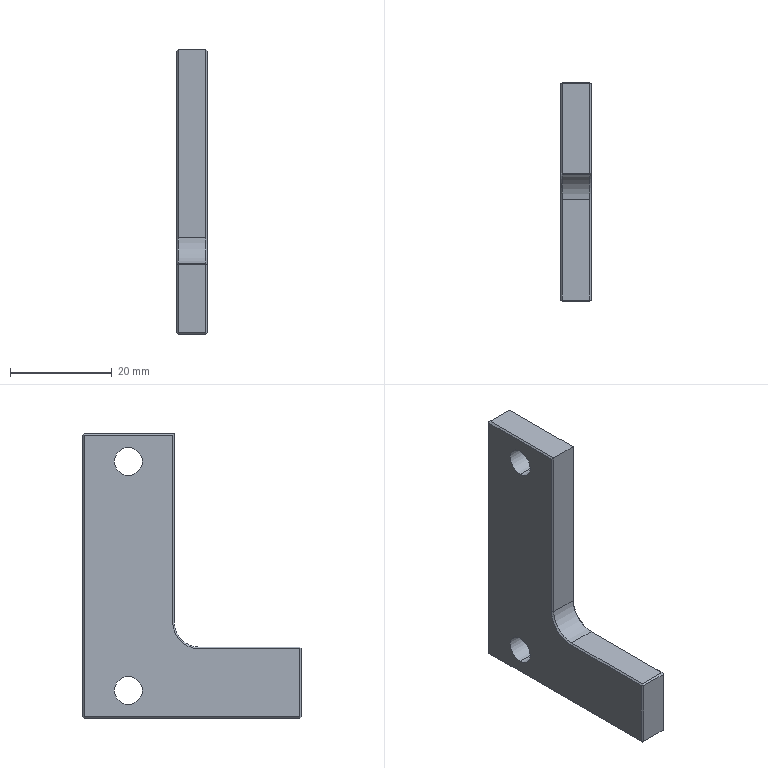Part | NX | 1 solid | 31 faces | box 6 x 43 x 56 mm | volume 7877 mm3 | plane 24 | cylinder 5 | cone 2 | commonest cylinder face diameters 5.5 x4 10 x1
STEP:
#1=CARTESIAN_POINT('',(2321.8,254.1,-75.2));
#2=VERTEX_POINT('',#1);
#3=CARTESIAN_POINT('',(2327.2,254.1,-75.2));
#4=VERTEX_POINT('',#3);
#5=CARTESIAN_POINT('',(2324.5,254.1,-75.2));
#6=DIRECTION('',(1.,0.,0.));
#7=VECTOR('',#6,1000.);
#8=LINE('',#5,#7);
#9=EDGE_CURVE('',#2,#4,#8,.T.);
#10=ORIENTED_EDGE('',*,*,#9,.T.);
#11=CARTESIAN_POINT('',(2327.2,211.7,-75.2));
#12=VERTEX_POINT('',#11);
#13=CARTESIAN_POINT('',(2327.2,232.9,-75.2));
#14=DIRECTION('',(0.,1.,0.));
#15=VECTOR('',#14,1000.);
#16=LINE('',#13,#15);
#17=EDGE_CURVE('',#12,#4,#16,.T.);
#18=ORIENTED_EDGE('',*,*,#17,.F.);
#19=CARTESIAN_POINT('',(2321.8,211.7,-75.2));
#20=VERTEX_POINT('',#19);
#21=CARTESIAN_POINT('',(2324.5,211.7,-75.2));
#22=DIRECTION('',(-1.,0.,0.));
#23=VECTOR('',#22,1000.);
#24=LINE('',#21,#23);
#25=EDGE_CURVE('',#12,#20,#24,.T.);
#26=ORIENTED_EDGE('',*,*,#25,.T.);
#27=CARTESIAN_POINT('',(2321.8,232.9,-75.2));
#28=DIRECTION('',(0.,1.,0.));
#29=VECTOR('',#28,1000.);
#30=LINE('',#27,#29);
#31=EDGE_CURVE('',#20,#2,#30,.T.);
#32=ORIENTED_EDGE('',*,*,#31,.T.);
#33=EDGE_LOOP('',(#10,#18,#26,#32));
#34=FACE_BOUND('',#33,.T.);
#35=CARTESIAN_POINT('',(2321.5,254.4,-75.2));
#36=DIRECTION('',(0.,0.,-1.));
#37=DIRECTION('',(-1.,0.,0.));
#38=AXIS2_PLACEMENT_3D('',#35,#36,#37);
#39=PLANE('',#38);
#40=ADVANCED_FACE('',(#34),#39,.T.);
#41=CARTESIAN_POINT('',(2321.8,254.4,-19.5));
#42=VERTEX_POINT('',#41);
#43=CARTESIAN_POINT('',(2327.2,254.4,-19.5));
#44=VERTEX_POINT('',#43);
#45=CARTESIAN_POINT('',(2324.5,254.4,-19.5));
#46=DIRECTION('',(1.,0.,0.));
#47=VECTOR('',#46,1000.);
#48=LINE('',#45,#47);
#49=EDGE_CURVE('',#42,#44,#48,.T.);
#50=ORIENTED_EDGE('',*,*,#49,.T.);
#51=CARTESIAN_POINT('',(2327.2,254.4,-74.9));
#52=VERTEX_POINT('',#51);
#53=CARTESIAN_POINT('',(2327.2,254.4,-47.2));
#54=DIRECTION('',(0.,0.,1.));
#55=VECTOR('',#54,1000.);
#56=LINE('',#53,#55);
#57=EDGE_CURVE('',#52,#44,#56,.T.);
#58=ORIENTED_EDGE('',*,*,#57,.F.);
#59=CARTESIAN_POINT('',(2321.8,254.4,-74.9));
#60=VERTEX_POINT('',#59);
#61=CARTESIAN_POINT('',(2324.5,254.4,-74.9));
#62=DIRECTION('',(1.,0.,0.));
#63=VECTOR('',#62,1000.);
#64=LINE('',#61,#63);
#65=EDGE_CURVE('',#60,#52,#64,.T.);
#66=ORIENTED_EDGE('',*,*,#65,.F.);
#67=CARTESIAN_POINT('',(2321.8,254.4,-47.2));
#68=DIRECTION('',(0.,0.,1.));
#69=VECTOR('',#68,1000.);
#70=LINE('',#67,#69);
#71=EDGE_CURVE('',#60,#42,#70,.T.);
#72=ORIENTED_EDGE('',*,*,#71,.T.);
#73=EDGE_LOOP('',(#50,#58,#66,#72));
#74=FACE_BOUND('',#73,.T.);
#75=CARTESIAN_POINT('',(2321.5,254.4,-19.2));
#76=DIRECTION('',(0.,1.,0.));
#77=DIRECTION('',(1.,0.,0.));
#78=AXIS2_PLACEMENT_3D('',#75,#76,#77);
#79=PLANE('',#78);
#80=ADVANCED_FACE('',(#74),#79,.T.);
#81=CARTESIAN_POINT('',(2321.8,254.1,-19.2));
#82=VERTEX_POINT('',#81);
#83=CARTESIAN_POINT('',(2321.8,236.4,-19.2));
#84=VERTEX_POINT('',#83);
#85=CARTESIAN_POINT('',(2321.8,245.4,-19.2));
#86=DIRECTION('',(0.,-1.,0.));
#87=VECTOR('',#86,1000.);
#88=LINE('',#85,#87);
#89=EDGE_CURVE('',#82,#84,#88,.T.);
#90=ORIENTED_EDGE('',*,*,#89,.T.);
#91=CARTESIAN_POINT('',(2327.2,236.4,-19.2));
#92=VERTEX_POINT('',#91);
#93=CARTESIAN_POINT('',(2321.5,236.4,-19.2));
#94=DIRECTION('',(1.,0.,0.));
#95=VECTOR('',#94,1000.);
#96=LINE('',#93,#95);
#97=EDGE_CURVE('',#84,#92,#96,.T.);
#98=ORIENTED_EDGE('',*,*,#97,.T.);
#99=CARTESIAN_POINT('',(2327.2,254.1,-19.2));
#100=VERTEX_POINT('',#99);
#101=CARTESIAN_POINT('',(2327.2,245.4,-19.2));
#102=DIRECTION('',(0.,-1.,0.));
#103=VECTOR('',#102,1000.);
#104=LINE('',#101,#103);
#105=EDGE_CURVE('',#100,#92,#104,.T.);
#106=ORIENTED_EDGE('',*,*,#105,.F.);
#107=CARTESIAN_POINT('',(2324.5,254.1,-19.2));
#108=DIRECTION('',(1.,0.,0.));
#109=VECTOR('',#108,1000.);
#110=LINE('',#107,#109);
#111=EDGE_CURVE('',#82,#100,#110,.T.);
#112=ORIENTED_EDGE('',*,*,#111,.F.);
#113=EDGE_LOOP('',(#90,#98,#106,#112));
#114=FACE_BOUND('',#113,.T.);
#115=CARTESIAN_POINT('',(2321.5,236.4,-19.2));
#116=DIRECTION('',(0.,0.,1.));
#117=DIRECTION('',(1.,0.,0.));
#118=AXIS2_PLACEMENT_3D('',#115,#116,#117);
#119=PLANE('',#118);
#120=ADVANCED_FACE('',(#114),#119,.T.);
#121=CARTESIAN_POINT('',(2327.2,236.4,-56.2));
#122=VERTEX_POINT('',#121);
#123=CARTESIAN_POINT('',(2321.8,236.4,-56.2));
#124=VERTEX_POINT('',#123);
#125=CARTESIAN_POINT('',(2321.5,236.4,-56.2));
#126=DIRECTION('',(-1.,0.,0.));
#127=VECTOR('',#126,1000.);
#128=LINE('',#125,#127);
#129=EDGE_CURVE('',#122,#124,#128,.T.);
#130=ORIENTED_EDGE('',*,*,#129,.F.);
#131=CARTESIAN_POINT('',(2327.2,236.4,-37.7));
#132=DIRECTION('',(0.,0.,-1.));
#133=VECTOR('',#132,1000.);
#134=LINE('',#131,#133);
#135=EDGE_CURVE('',#92,#122,#134,.T.);
#136=ORIENTED_EDGE('',*,*,#135,.F.);
#137=ORIENTED_EDGE('',*,*,#97,.F.);
#138=CARTESIAN_POINT('',(2321.8,236.4,-37.7));
#139=DIRECTION('',(0.,0.,-1.));
#140=VECTOR('',#139,1000.);
#141=LINE('',#138,#140);
#142=EDGE_CURVE('',#84,#124,#141,.T.);
#143=ORIENTED_EDGE('',*,*,#142,.T.);
#144=EDGE_LOOP('',(#130,#136,#137,#143));
#145=FACE_BOUND('',#144,.T.);
#146=CARTESIAN_POINT('',(2321.5,236.4,-75.2));
#147=DIRECTION('',(0.,-1.,0.));
#148=DIRECTION('',(0.,0.,-1.));
#149=AXIS2_PLACEMENT_3D('',#146,#147,#148);
#150=PLANE('',#149);
#151=ADVANCED_FACE('',(#145),#150,.T.);
#152=CARTESIAN_POINT('',(2327.2,211.4,-74.9));
#153=VERTEX_POINT('',#152);
#154=CARTESIAN_POINT('',(2321.8,211.4,-74.9));
#155=VERTEX_POINT('',#154);
#156=CARTESIAN_POINT('',(2324.5,211.4,-74.9));
#157=DIRECTION('',(-1.,0.,0.));
#158=VECTOR('',#157,1000.);
#159=LINE('',#156,#158);
#160=EDGE_CURVE('',#153,#155,#159,.T.);
#161=ORIENTED_EDGE('',*,*,#160,.F.);
#162=CARTESIAN_POINT('',(2327.2,211.4,-61.5));
#163=VERTEX_POINT('',#162);
#164=CARTESIAN_POINT('',(2327.2,211.4,-68.2));
#165=DIRECTION('',(0.,0.,-1.));
#166=VECTOR('',#165,1000.);
#167=LINE('',#164,#166);
#168=EDGE_CURVE('',#163,#153,#167,.T.);
#169=ORIENTED_EDGE('',*,*,#168,.F.);
#170=CARTESIAN_POINT('',(2321.8,211.4,-61.5));
#171=VERTEX_POINT('',#170);
#172=CARTESIAN_POINT('',(2324.5,211.4,-61.5));
#173=DIRECTION('',(1.,0.,0.));
#174=VECTOR('',#173,1000.);
#175=LINE('',#172,#174);
#176=EDGE_CURVE('',#171,#163,#175,.T.);
#177=ORIENTED_EDGE('',*,*,#176,.F.);
#178=CARTESIAN_POINT('',(2321.8,211.4,-68.2));
#179=DIRECTION('',(0.,0.,-1.));
#180=VECTOR('',#179,1000.);
#181=LINE('',#178,#180);
#182=EDGE_CURVE('',#171,#155,#181,.T.);
#183=ORIENTED_EDGE('',*,*,#182,.T.);
#184=EDGE_LOOP('',(#161,#169,#177,#183));
#185=FACE_BOUND('',#184,.T.);
#186=CARTESIAN_POINT('',(2325.077,211.4,-68.526));
#187=DIRECTION('',(0.,-1.,0.));
#188=DIRECTION('',(0.,0.,-1.));
#189=AXIS2_PLACEMENT_3D('',#186,#187,#188);
#190=PLANE('',#189);
#191=ADVANCED_FACE('',(#185),#190,.T.);
#192=CARTESIAN_POINT('',(2321.8,231.4,-61.2));
#193=VERTEX_POINT('',#192);
#194=CARTESIAN_POINT('',(2321.8,211.7,-61.2));
#195=VERTEX_POINT('',#194);
#196=CARTESIAN_POINT('',(2321.8,221.4,-61.2));
#197=DIRECTION('',(0.,-1.,0.));
#198=VECTOR('',#197,1000.);
#199=LINE('',#196,#198);
#200=EDGE_CURVE('',#193,#195,#199,.T.);
#201=ORIENTED_EDGE('',*,*,#200,.T.);
#202=CARTESIAN_POINT('',(2327.2,211.7,-61.2));
#203=VERTEX_POINT('',#202);
#204=CARTESIAN_POINT('',(2324.5,211.7,-61.2));
#205=DIRECTION('',(1.,0.,0.));
#206=VECTOR('',#205,1000.);
#207=LINE('',#204,#206);
#208=EDGE_CURVE('',#195,#203,#207,.T.);
#209=ORIENTED_EDGE('',*,*,#208,.T.);
#210=CARTESIAN_POINT('',(2327.2,231.4,-61.2));
#211=VERTEX_POINT('',#210);
#212=CARTESIAN_POINT('',(2327.2,221.4,-61.2));
#213=DIRECTION('',(0.,-1.,0.));
#214=VECTOR('',#213,1000.);
#215=LINE('',#212,#214);
#216=EDGE_CURVE('',#211,#203,#215,.T.);
#217=ORIENTED_EDGE('',*,*,#216,.F.);
#218=CARTESIAN_POINT('',(2321.5,231.4,-61.2));
#219=DIRECTION('',(-1.,0.,0.));
#220=VECTOR('',#219,1000.);
#221=LINE('',#218,#220);
#222=EDGE_CURVE('',#211,#193,#221,.T.);
#223=ORIENTED_EDGE('',*,*,#222,.T.);
#224=EDGE_LOOP('',(#201,#209,#217,#223));
#225=FACE_BOUND('',#224,.T.);
#226=CARTESIAN_POINT('',(2321.5,236.4,-61.2));
#227=DIRECTION('',(0.,0.,1.));
#228=DIRECTION('',(1.,0.,0.));
#229=AXIS2_PLACEMENT_3D('',#226,#227,#228);
#230=PLANE('',#229);
#231=ADVANCED_FACE('',(#225),#230,.T.);
#232=CARTESIAN_POINT('',(2321.8,231.4,-56.2));
#233=DIRECTION('',(-1.,0.,0.));
#234=DIRECTION('',(0.,0.,-1.));
#235=AXIS2_PLACEMENT_3D('',#232,#233,#234);
#236=CIRCLE('',#235,5.);
#237=EDGE_CURVE('',#124,#193,#236,.T.);
#238=ORIENTED_EDGE('',*,*,#237,.T.);
#239=ORIENTED_EDGE('',*,*,#222,.F.);
#240=CARTESIAN_POINT('',(2327.2,231.4,-56.2));
#241=DIRECTION('',(-1.,0.,0.));
#242=DIRECTION('',(0.,0.,-1.));
#243=AXIS2_PLACEMENT_3D('',#240,#241,#242);
#244=CIRCLE('',#243,5.);
#245=EDGE_CURVE('',#122,#211,#244,.T.);
#246=ORIENTED_EDGE('',*,*,#245,.F.);
#247=ORIENTED_EDGE('',*,*,#129,.T.);
#248=EDGE_LOOP('',(#238,#239,#246,#247));
#249=FACE_BOUND('',#248,.T.);
#250=CARTESIAN_POINT('',(2321.5,231.4,-56.2));
#251=DIRECTION('',(-1.,0.,0.));
#252=DIRECTION('',(0.,0.,-1.));
#253=AXIS2_PLACEMENT_3D('',#250,#251,#252);
#254=CYLINDRICAL_SURFACE('',#253,5.);
#255=ADVANCED_FACE('',(#249),#254,.F.);
#256=ORIENTED_EDGE('',*,*,#49,.F.);
#257=CARTESIAN_POINT('',(2321.65,254.25,-19.35));
#258=VERTEX_POINT('',#257);
#259=CARTESIAN_POINT('',(2347.565,280.165,-45.265));
#260=DIRECTION('',(0.5774,0.5774,-0.5774));
#261=VECTOR('',#260,1000.);
#262=LINE('',#259,#261);
#263=EDGE_CURVE('',#258,#42,#262,.T.);
#264=ORIENTED_EDGE('',*,*,#263,.F.);
#265=CARTESIAN_POINT('',(2295.735,280.165,-45.265));
#266=DIRECTION('',(0.5774,-0.5774,0.5774));
#267=VECTOR('',#266,1000.);
#268=LINE('',#265,#267);
#269=EDGE_CURVE('',#258,#82,#268,.T.);
#270=ORIENTED_EDGE('',*,*,#269,.T.);
#271=ORIENTED_EDGE('',*,*,#111,.T.);
#272=CARTESIAN_POINT('',(2327.35,254.25,-19.35));
#273=VERTEX_POINT('',#272);
#274=CARTESIAN_POINT('',(2353.265,280.165,-45.265));
#275=DIRECTION('',(-0.5774,-0.5774,0.5774));
#276=VECTOR('',#275,1000.);
#277=LINE('',#274,#276);
#278=EDGE_CURVE('',#273,#100,#277,.T.);
#279=ORIENTED_EDGE('',*,*,#278,.F.);
#280=CARTESIAN_POINT('',(2301.435,280.165,-45.265));
#281=DIRECTION('',(-0.5774,0.5774,-0.5774));
#282=VECTOR('',#281,1000.);
#283=LINE('',#280,#282);
#284=EDGE_CURVE('',#273,#44,#283,.T.);
#285=ORIENTED_EDGE('',*,*,#284,.T.);
#286=EDGE_LOOP('',(#256,#264,#270,#271,#279,#285));
#287=FACE_BOUND('',#286,.T.);
#288=CARTESIAN_POINT('',(2324.5,254.25,-19.35));
#289=DIRECTION('',(0.,0.7071,0.7071));
#290=DIRECTION('',(1.,0.,0.));
#291=AXIS2_PLACEMENT_3D('',#288,#289,#290);
#292=PLANE('',#291);
#293=ADVANCED_FACE('',(#287),#292,.T.);
#294=ORIENTED_EDGE('',*,*,#9,.F.);
#295=CARTESIAN_POINT('',(2321.65,254.25,-75.05));
#296=VERTEX_POINT('',#295);
#297=CARTESIAN_POINT('',(2329.326,246.574,-82.726));
#298=DIRECTION('',(0.5774,-0.5774,-0.5774));
#299=VECTOR('',#298,1000.);
#300=LINE('',#297,#299);
#301=EDGE_CURVE('',#296,#2,#300,.T.);
#302=ORIENTED_EDGE('',*,*,#301,.F.);
#303=CARTESIAN_POINT('',(2321.5,254.1,-75.2));
#304=DIRECTION('',(0.5774,0.5774,0.5774));
#305=VECTOR('',#304,1000.);
#306=LINE('',#303,#305);
#307=EDGE_CURVE('',#296,#60,#306,.T.);
#308=ORIENTED_EDGE('',*,*,#307,.T.);
#309=ORIENTED_EDGE('',*,*,#65,.T.);
#310=CARTESIAN_POINT('',(2327.35,254.25,-75.05));
#311=VERTEX_POINT('',#310);
#312=CARTESIAN_POINT('',(2321.5,260.1,-69.2));
#313=DIRECTION('',(-0.5774,0.5774,0.5774));
#314=VECTOR('',#313,1000.);
#315=LINE('',#312,#314);
#316=EDGE_CURVE('',#311,#52,#315,.T.);
#317=ORIENTED_EDGE('',*,*,#316,.F.);
#318=CARTESIAN_POINT('',(2319.674,246.574,-82.726));
#319=DIRECTION('',(-0.5774,-0.5774,-0.5774));
#320=VECTOR('',#319,1000.);
#321=LINE('',#318,#320);
#322=EDGE_CURVE('',#311,#4,#321,.T.);
#323=ORIENTED_EDGE('',*,*,#322,.T.);
#324=EDGE_LOOP('',(#294,#302,#308,#309,#317,#323));
#325=FACE_BOUND('',#324,.T.);
#326=CARTESIAN_POINT('',(2324.5,254.25,-75.05));
#327=DIRECTION('',(0.,0.7071,-0.7071));
#328=DIRECTION('',(-1.,0.,0.));
#329=AXIS2_PLACEMENT_3D('',#326,#327,#328);
#330=PLANE('',#329);
#331=ADVANCED_FACE('',(#325),#330,.T.);
#332=ORIENTED_EDGE('',*,*,#168,.T.);
#333=CARTESIAN_POINT('',(2327.35,211.55,-75.05));
#334=VERTEX_POINT('',#333);
#335=CARTESIAN_POINT('',(2297.565,181.765,-45.265));
#336=DIRECTION('',(0.5774,0.5774,-0.5774));
#337=VECTOR('',#336,1000.);
#338=LINE('',#335,#337);
#339=EDGE_CURVE('',#153,#334,#338,.T.);
#340=ORIENTED_EDGE('',*,*,#339,.T.);
#341=CARTESIAN_POINT('',(2327.5,211.7,-74.9));
#342=VERTEX_POINT('',#341);
#343=CARTESIAN_POINT('',(2357.135,241.335,-45.265));
#344=DIRECTION('',(0.5774,0.5774,0.5774));
#345=VECTOR('',#344,1000.);
#346=LINE('',#343,#345);
#347=EDGE_CURVE('',#334,#342,#346,.T.);
#348=ORIENTED_EDGE('',*,*,#347,.T.);
#349=CARTESIAN_POINT('',(2327.5,211.7,-61.5));
#350=VERTEX_POINT('',#349);
#351=CARTESIAN_POINT('',(2327.5,211.7,-68.2));
#352=DIRECTION('',(0.,0.,-1.));
#353=VECTOR('',#352,1000.);
#354=LINE('',#351,#353);
#355=EDGE_CURVE('',#350,#342,#354,.T.);
#356=ORIENTED_EDGE('',*,*,#355,.F.);
#357=CARTESIAN_POINT('',(2327.35,211.55,-61.35));
#358=VERTEX_POINT('',#357);
#359=CARTESIAN_POINT('',(2311.265,195.465,-45.265));
#360=DIRECTION('',(0.5774,0.5774,-0.5774));
#361=VECTOR('',#360,1000.);
#362=LINE('',#359,#361);
#363=EDGE_CURVE('',#358,#350,#362,.T.);
#364=ORIENTED_EDGE('',*,*,#363,.F.);
#365=CARTESIAN_POINT('',(2343.435,227.635,-45.265));
#366=DIRECTION('',(-0.5774,-0.5774,-0.5774));
#367=VECTOR('',#366,1000.);
#368=LINE('',#365,#367);
#369=EDGE_CURVE('',#358,#163,#368,.T.);
#370=ORIENTED_EDGE('',*,*,#369,.T.);
#371=EDGE_LOOP('',(#332,#340,#348,#356,#364,#370));
#372=FACE_BOUND('',#371,.T.);
#373=CARTESIAN_POINT('',(2327.35,211.55,-68.2));
#374=DIRECTION('',(-0.7071,0.7071,0.));
#375=DIRECTION('',(0.,0.,1.));
#376=AXIS2_PLACEMENT_3D('',#373,#374,#375);
#377=PLANE('',#376);
#378=ADVANCED_FACE('',(#372),#377,.F.);
#379=ORIENTED_EDGE('',*,*,#245,.T.);
#380=CARTESIAN_POINT('',(2327.5,231.4,-61.5));
#381=VERTEX_POINT('',#380);
#382=CARTESIAN_POINT('',(2327.5,231.4,-61.5));
#383=DIRECTION('',(-0.7071,0.,0.7071));
#384=VECTOR('',#383,1000.);
#385=LINE('',#382,#384);
#386=EDGE_CURVE('',#381,#211,#385,.T.);
#387=ORIENTED_EDGE('',*,*,#386,.F.);
#388=CARTESIAN_POINT('',(2327.5,236.7,-56.2));
#389=VERTEX_POINT('',#388);
#390=CARTESIAN_POINT('',(2327.5,231.4,-56.2));
#391=DIRECTION('',(-1.,0.,0.));
#392=DIRECTION('',(0.,0.,-1.));
#393=AXIS2_PLACEMENT_3D('',#390,#391,#392);
#394=CIRCLE('',#393,5.3);
#395=EDGE_CURVE('',#389,#381,#394,.T.);
#396=ORIENTED_EDGE('',*,*,#395,.F.);
#397=CARTESIAN_POINT('',(2327.2,236.4,-56.2));
#398=DIRECTION('',(0.7071,0.7071,0.));
#399=VECTOR('',#398,1000.);
#400=LINE('',#397,#399);
#401=EDGE_CURVE('',#122,#389,#400,.T.);
#402=ORIENTED_EDGE('',*,*,#401,.F.);
#403=EDGE_LOOP('',(#379,#387,#396,#402));
#404=FACE_BOUND('',#403,.T.);
#405=CARTESIAN_POINT('',(2327.2,231.4,-56.2));
#406=DIRECTION('',(1.,0.,0.));
#407=DIRECTION('',(0.,-1.,0.));
#408=AXIS2_PLACEMENT_3D('',#405,#406,#407);
#409=CONICAL_SURFACE('',#408,5.,0.7854);
#410=ADVANCED_FACE('',(#404),#409,.F.);
#411=ORIENTED_EDGE('',*,*,#200,.F.);
#412=CARTESIAN_POINT('',(2321.5,231.4,-61.5));
#413=VERTEX_POINT('',#412);
#414=CARTESIAN_POINT('',(2321.8,231.4,-61.2));
#415=DIRECTION('',(-0.7071,0.,-0.7071));
#416=VECTOR('',#415,1000.);
#417=LINE('',#414,#416);
#418=EDGE_CURVE('',#193,#413,#417,.T.);
#419=ORIENTED_EDGE('',*,*,#418,.T.);
#420=CARTESIAN_POINT('',(2321.5,211.7,-61.5));
#421=VERTEX_POINT('',#420);
#422=CARTESIAN_POINT('',(2321.5,221.4,-61.5));
#423=DIRECTION('',(0.,-1.,0.));
#424=VECTOR('',#423,1000.);
#425=LINE('',#422,#424);
#426=EDGE_CURVE('',#413,#421,#425,.T.);
#427=ORIENTED_EDGE('',*,*,#426,.T.);
#428=CARTESIAN_POINT('',(2321.65,211.55,-61.35));
#429=VERTEX_POINT('',#428);
#430=CARTESIAN_POINT('',(2337.735,195.465,-45.265));
#431=DIRECTION('',(0.5774,-0.5774,0.5774));
#432=VECTOR('',#431,1000.);
#433=LINE('',#430,#432);
#434=EDGE_CURVE('',#421,#429,#433,.T.);
#435=ORIENTED_EDGE('',*,*,#434,.T.);
#436=CARTESIAN_POINT('',(2337.735,227.635,-45.265));
#437=DIRECTION('',(-0.5774,-0.5774,-0.5774));
#438=VECTOR('',#437,1000.);
#439=LINE('',#436,#438);
#440=EDGE_CURVE('',#195,#429,#439,.T.);
#441=ORIENTED_EDGE('',*,*,#440,.F.);
#442=EDGE_LOOP('',(#411,#419,#427,#435,#441));
#443=FACE_BOUND('',#442,.T.);
#444=CARTESIAN_POINT('',(2321.65,221.4,-61.35));
#445=DIRECTION('',(-0.7071,0.,0.7071));
#446=DIRECTION('',(0.,1.,0.));
#447=AXIS2_PLACEMENT_3D('',#444,#445,#446);
#448=PLANE('',#447);
#449=ADVANCED_FACE('',(#443),#448,.T.);
#450=ORIENTED_EDGE('',*,*,#237,.F.);
#451=CARTESIAN_POINT('',(2321.5,236.7,-56.2));
#452=VERTEX_POINT('',#451);
#453=CARTESIAN_POINT('',(2321.8,236.4,-56.2));
#454=DIRECTION('',(-0.7071,0.7071,0.));
#455=VECTOR('',#454,1000.);
#456=LINE('',#453,#455);
#457=EDGE_CURVE('',#124,#452,#456,.T.);
#458=ORIENTED_EDGE('',*,*,#457,.T.);
#459=CARTESIAN_POINT('',(2321.5,231.4,-56.2));
#460=DIRECTION('',(-1.,0.,0.));
#461=DIRECTION('',(0.,0.,-1.));
#462=AXIS2_PLACEMENT_3D('',#459,#460,#461);
#463=CIRCLE('',#462,5.3);
#464=EDGE_CURVE('',#452,#413,#463,.T.);
#465=ORIENTED_EDGE('',*,*,#464,.T.);
#466=ORIENTED_EDGE('',*,*,#418,.F.);
#467=EDGE_LOOP('',(#450,#458,#465,#466));
#468=FACE_BOUND('',#467,.T.);
#469=CARTESIAN_POINT('',(2321.8,231.4,-56.2));
#470=DIRECTION('',(-1.,0.,0.));
#471=DIRECTION('',(0.,1.,0.));
#472=AXIS2_PLACEMENT_3D('',#469,#470,#471);
#473=CONICAL_SURFACE('',#472,5.,0.7854);
#474=ADVANCED_FACE('',(#468),#473,.F.);
#475=ORIENTED_EDGE('',*,*,#176,.T.);
#476=ORIENTED_EDGE('',*,*,#369,.F.);
#477=CARTESIAN_POINT('',(2311.265,227.635,-45.265));
#478=DIRECTION('',(-0.5774,0.5774,0.5774));
#479=VECTOR('',#478,1000.);
#480=LINE('',#477,#479);
#481=EDGE_CURVE('',#358,#203,#480,.T.);
#482=ORIENTED_EDGE('',*,*,#481,.T.);
#483=ORIENTED_EDGE('',*,*,#208,.F.);
#484=ORIENTED_EDGE('',*,*,#440,.T.);
#485=CARTESIAN_POINT('',(2305.565,227.635,-45.265));
#486=DIRECTION('',(-0.5774,0.5774,0.5774));
#487=VECTOR('',#486,1000.);
#488=LINE('',#485,#487);
#489=EDGE_CURVE('',#171,#429,#488,.T.);
#490=ORIENTED_EDGE('',*,*,#489,.F.);
#491=EDGE_LOOP('',(#475,#476,#482,#483,#484,#490));
#492=FACE_BOUND('',#491,.T.);
#493=CARTESIAN_POINT('',(2324.5,211.55,-61.35));
#494=DIRECTION('',(0.,0.7071,-0.7071));
#495=DIRECTION('',(-1.,0.,0.));
#496=AXIS2_PLACEMENT_3D('',#493,#494,#495);
#497=PLANE('',#496);
#498=ADVANCED_FACE('',(#492),#497,.F.);
#499=ORIENTED_EDGE('',*,*,#182,.F.);
#500=ORIENTED_EDGE('',*,*,#489,.T.);
#501=ORIENTED_EDGE('',*,*,#434,.F.);
#502=CARTESIAN_POINT('',(2321.5,211.7,-74.9));
#503=VERTEX_POINT('',#502);
#504=CARTESIAN_POINT('',(2321.5,211.7,-68.2));
#505=DIRECTION('',(0.,0.,-1.));
#506=VECTOR('',#505,1000.);
#507=LINE('',#504,#506);
#508=EDGE_CURVE('',#421,#503,#507,.T.);
#509=ORIENTED_EDGE('',*,*,#508,.T.);
#510=CARTESIAN_POINT('',(2321.65,211.55,-75.05));
#511=VERTEX_POINT('',#510);
#512=CARTESIAN_POINT('',(2291.865,241.335,-45.265));
#513=DIRECTION('',(-0.5774,0.5774,0.5774));
#514=VECTOR('',#513,1000.);
#515=LINE('',#512,#514);
#516=EDGE_CURVE('',#511,#503,#515,.T.);
#517=ORIENTED_EDGE('',*,*,#516,.F.);
#518=CARTESIAN_POINT('',(2351.435,181.765,-45.265));
#519=DIRECTION('',(-0.5774,0.5774,-0.5774));
#520=VECTOR('',#519,1000.);
#521=LINE('',#518,#520);
#522=EDGE_CURVE('',#155,#511,#521,.T.);
#523=ORIENTED_EDGE('',*,*,#522,.F.);
#524=EDGE_LOOP('',(#499,#500,#501,#509,#517,#523));
#525=FACE_BOUND('',#524,.T.);
#526=CARTESIAN_POINT('',(2321.65,211.55,-68.2));
#527=DIRECTION('',(-0.7071,-0.7071,0.));
#528=DIRECTION('',(-0.7071,0.7071,0.));
#529=AXIS2_PLACEMENT_3D('',#526,#527,#528);
#530=PLANE('',#529);
#531=ADVANCED_FACE('',(#525),#530,.T.);
#532=ORIENTED_EDGE('',*,*,#160,.T.);
#533=ORIENTED_EDGE('',*,*,#522,.T.);
#534=CARTESIAN_POINT('',(2291.865,181.765,-45.265));
#535=DIRECTION('',(-0.5774,-0.5774,0.5774));
#536=VECTOR('',#535,1000.);
#537=LINE('',#534,#536);
#538=EDGE_CURVE('',#20,#511,#537,.T.);
#539=ORIENTED_EDGE('',*,*,#538,.F.);
#540=ORIENTED_EDGE('',*,*,#25,.F.);
#541=CARTESIAN_POINT('',(2357.135,181.765,-45.265));
#542=DIRECTION('',(0.5774,-0.5774,0.5774));
#543=VECTOR('',#542,1000.);
#544=LINE('',#541,#543);
#545=EDGE_CURVE('',#12,#334,#544,.T.);
#546=ORIENTED_EDGE('',*,*,#545,.T.);
#547=ORIENTED_EDGE('',*,*,#339,.F.);
#548=EDGE_LOOP('',(#532,#533,#539,#540,#546,#547));
#549=FACE_BOUND('',#548,.T.);
#550=CARTESIAN_POINT('',(2324.5,211.55,-75.05));
#551=DIRECTION('',(0.,0.7071,0.7071));
#552=DIRECTION('',(1.,0.,0.));
#553=AXIS2_PLACEMENT_3D('',#550,#551,#552);
#554=PLANE('',#553);
#555=ADVANCED_FACE('',(#549),#554,.F.);
#556=CARTESIAN_POINT('',(2327.5,236.7,-19.5));
#557=VERTEX_POINT('',#556);
#558=CARTESIAN_POINT('',(2327.5,236.7,-37.7));
#559=DIRECTION('',(0.,0.,-1.));
#560=VECTOR('',#559,1000.);
#561=LINE('',#558,#560);
#562=EDGE_CURVE('',#557,#389,#561,.T.);
#563=ORIENTED_EDGE('',*,*,#562,.T.);
#564=ORIENTED_EDGE('',*,*,#395,.T.);
#565=CARTESIAN_POINT('',(2327.5,221.4,-61.5));
#566=DIRECTION('',(0.,-1.,0.));
#567=VECTOR('',#566,1000.);
#568=LINE('',#565,#567);
#569=EDGE_CURVE('',#381,#350,#568,.T.);
#570=ORIENTED_EDGE('',*,*,#569,.T.);
#571=ORIENTED_EDGE('',*,*,#355,.T.);
#572=CARTESIAN_POINT('',(2327.5,254.1,-74.9));
#573=VERTEX_POINT('',#572);
#574=CARTESIAN_POINT('',(2327.5,232.9,-74.9));
#575=DIRECTION('',(0.,1.,0.));
#576=VECTOR('',#575,1000.);
#577=LINE('',#574,#576);
#578=EDGE_CURVE('',#342,#573,#577,.T.);
#579=ORIENTED_EDGE('',*,*,#578,.T.);
#580=CARTESIAN_POINT('',(2327.5,254.1,-19.5));
#581=VERTEX_POINT('',#580);
#582=CARTESIAN_POINT('',(2327.5,254.1,-47.2));
#583=DIRECTION('',(0.,0.,1.));
#584=VECTOR('',#583,1000.);
#585=LINE('',#582,#584);
#586=EDGE_CURVE('',#573,#581,#585,.T.);
#587=ORIENTED_EDGE('',*,*,#586,.T.);
#588=CARTESIAN_POINT('',(2327.5,245.4,-19.5));
#589=DIRECTION('',(0.,-1.,0.));
#590=VECTOR('',#589,1000.);
#591=LINE('',#588,#590);
#592=EDGE_CURVE('',#581,#557,#591,.T.);
#593=ORIENTED_EDGE('',*,*,#592,.T.);
#594=EDGE_LOOP('',(#563,#564,#570,#571,#579,#587,#593));
#595=FACE_BOUND('',#594,.T.);
#596=CARTESIAN_POINT('',(2327.5,245.4,-66.95));
#597=VERTEX_POINT('',#596);
#598=CARTESIAN_POINT('',(2327.5,245.4,-72.45));
#599=VERTEX_POINT('',#598);
#600=CARTESIAN_POINT('',(2327.5,245.4,-69.7));
#601=DIRECTION('',(1.,0.,0.));
#602=DIRECTION('',(0.,0.,-1.));
#603=AXIS2_PLACEMENT_3D('',#600,#601,#602);
#604=CIRCLE('',#603,2.75);
#605=EDGE_CURVE('',#597,#599,#604,.T.);
#606=ORIENTED_EDGE('',*,*,#605,.F.);
#607=CARTESIAN_POINT('',(2327.5,245.4,-69.7));
#608=DIRECTION('',(1.,0.,0.));
#609=DIRECTION('',(0.,0.,-1.));
#610=AXIS2_PLACEMENT_3D('',#607,#608,#609);
#611=CIRCLE('',#610,2.75);
#612=EDGE_CURVE('',#599,#597,#611,.T.);
#613=ORIENTED_EDGE('',*,*,#612,.F.);
#614=EDGE_LOOP('',(#606,#613));
#615=FACE_BOUND('',#614,.T.);
#616=CARTESIAN_POINT('',(2327.5,245.4,-27.45));
#617=VERTEX_POINT('',#616);
#618=CARTESIAN_POINT('',(2327.5,245.4,-21.95));
#619=VERTEX_POINT('',#618);
#620=CARTESIAN_POINT('',(2327.5,245.4,-24.7));
#621=DIRECTION('',(1.,0.,0.));
#622=DIRECTION('',(0.,0.,-1.));
#623=AXIS2_PLACEMENT_3D('',#620,#621,#622);
#624=CIRCLE('',#623,2.75);
#625=EDGE_CURVE('',#617,#619,#624,.T.);
#626=ORIENTED_EDGE('',*,*,#625,.F.);
#627=CARTESIAN_POINT('',(2327.5,245.4,-24.7));
#628=DIRECTION('',(1.,0.,0.));
#629=DIRECTION('',(0.,0.,-1.));
#630=AXIS2_PLACEMENT_3D('',#627,#628,#629);
#631=CIRCLE('',#630,2.75);
#632=EDGE_CURVE('',#619,#617,#631,.T.);
#633=ORIENTED_EDGE('',*,*,#632,.F.);
#634=EDGE_LOOP('',(#626,#633));
#635=FACE_BOUND('',#634,.T.);
#636=CARTESIAN_POINT('',(2327.5,246.574,-45.265));
#637=DIRECTION('',(1.,0.,0.));
#638=DIRECTION('',(0.,1.,0.));
#639=AXIS2_PLACEMENT_3D('',#636,#637,#638);
#640=PLANE('',#639);
#641=ADVANCED_FACE('',(#595,#615,#635),#640,.T.);
#642=ORIENTED_EDGE('',*,*,#625,.T.);
#643=CARTESIAN_POINT('',(2321.5,245.4,-21.95));
#644=VERTEX_POINT('',#643);
#645=CARTESIAN_POINT('',(2320.9,245.4,-21.95));
#646=DIRECTION('',(1.,0.,0.));
#647=VECTOR('',#646,1000.);
#648=LINE('',#645,#647);
#649=EDGE_CURVE('',#644,#619,#648,.T.);
#650=ORIENTED_EDGE('',*,*,#649,.F.);
#651=CARTESIAN_POINT('',(2321.5,245.4,-27.45));
#652=VERTEX_POINT('',#651);
#653=CARTESIAN_POINT('',(2321.5,245.4,-24.7));
#654=DIRECTION('',(1.,0.,0.));
#655=DIRECTION('',(0.,0.,-1.));
#656=AXIS2_PLACEMENT_3D('',#653,#654,#655);
#657=CIRCLE('',#656,2.75);
#658=EDGE_CURVE('',#652,#644,#657,.T.);
#659=ORIENTED_EDGE('',*,*,#658,.F.);
#660=CARTESIAN_POINT('',(2320.9,245.4,-27.45));
#661=DIRECTION('',(1.,0.,0.));
#662=VECTOR('',#661,1000.);
#663=LINE('',#660,#662);
#664=EDGE_CURVE('',#652,#617,#663,.T.);
#665=ORIENTED_EDGE('',*,*,#664,.T.);
#666=EDGE_LOOP('',(#642,#650,#659,#665));
#667=FACE_BOUND('',#666,.T.);
#668=CARTESIAN_POINT('',(2320.9,245.4,-24.7));
#669=DIRECTION('',(1.,0.,0.));
#670=DIRECTION('',(0.,0.,-1.));
#671=AXIS2_PLACEMENT_3D('',#668,#669,#670);
#672=CYLINDRICAL_SURFACE('',#671,2.75);
#673=ADVANCED_FACE('',(#667),#672,.F.);
#674=CARTESIAN_POINT('',(2321.5,245.4,-66.95));
#675=VERTEX_POINT('',#674);
#676=CARTESIAN_POINT('',(2321.5,245.4,-72.45));
#677=VERTEX_POINT('',#676);
#678=CARTESIAN_POINT('',(2321.5,245.4,-69.7));
#679=DIRECTION('',(1.,0.,0.));
#680=DIRECTION('',(0.,0.,-1.));
#681=AXIS2_PLACEMENT_3D('',#678,#679,#680);
#682=CIRCLE('',#681,2.75);
#683=EDGE_CURVE('',#675,#677,#682,.T.);
#684=ORIENTED_EDGE('',*,*,#683,.F.);
#685=CARTESIAN_POINT('',(2320.9,245.4,-66.95));
#686=DIRECTION('',(1.,0.,0.));
#687=VECTOR('',#686,1000.);
#688=LINE('',#685,#687);
#689=EDGE_CURVE('',#675,#597,#688,.T.);
#690=ORIENTED_EDGE('',*,*,#689,.T.);
#691=ORIENTED_EDGE('',*,*,#605,.T.);
#692=CARTESIAN_POINT('',(2320.9,245.4,-72.45));
#693=DIRECTION('',(1.,0.,0.));
#694=VECTOR('',#693,1000.);
#695=LINE('',#692,#694);
#696=EDGE_CURVE('',#677,#599,#695,.T.);
#697=ORIENTED_EDGE('',*,*,#696,.F.);
#698=EDGE_LOOP('',(#684,#690,#691,#697));
#699=FACE_BOUND('',#698,.T.);
#700=CARTESIAN_POINT('',(2320.9,245.4,-69.7));
#701=DIRECTION('',(1.,0.,0.));
#702=DIRECTION('',(0.,0.,-1.));
#703=AXIS2_PLACEMENT_3D('',#700,#701,#702);
#704=CYLINDRICAL_SURFACE('',#703,2.75);
#705=ADVANCED_FACE('',(#699),#704,.F.);
#706=ORIENTED_EDGE('',*,*,#592,.F.);
#707=CARTESIAN_POINT('',(2353.265,228.335,-45.265));
#708=DIRECTION('',(-0.5774,0.5774,0.5774));
#709=VECTOR('',#708,1000.);
#710=LINE('',#707,#709);
#711=EDGE_CURVE('',#581,#273,#710,.T.);
#712=ORIENTED_EDGE('',*,*,#711,.T.);
#713=ORIENTED_EDGE('',*,*,#278,.T.);
#714=ORIENTED_EDGE('',*,*,#105,.T.);
#715=CARTESIAN_POINT('',(2353.265,262.465,-45.265));
#716=DIRECTION('',(0.5774,0.5774,-0.5774));
#717=VECTOR('',#716,1000.);
#718=LINE('',#715,#717);
#719=EDGE_CURVE('',#92,#557,#718,.T.);
#720=ORIENTED_EDGE('',*,*,#719,.T.);
#721=EDGE_LOOP('',(#706,#712,#713,#714,#720));
#722=FACE_BOUND('',#721,.T.);
#723=CARTESIAN_POINT('',(2327.35,245.4,-19.35));
#724=DIRECTION('',(0.7071,0.,0.7071));
#725=DIRECTION('',(0.,-1.,0.));
#726=AXIS2_PLACEMENT_3D('',#723,#724,#725);
#727=PLANE('',#726);
#728=ADVANCED_FACE('',(#722),#727,.T.);
#729=ORIENTED_EDGE('',*,*,#586,.F.);
#730=CARTESIAN_POINT('',(2357.135,224.465,-45.265));
#731=DIRECTION('',(-0.5774,0.5774,-0.5774));
#732=VECTOR('',#731,1000.);
#733=LINE('',#730,#732);
#734=EDGE_CURVE('',#573,#311,#733,.T.);
#735=ORIENTED_EDGE('',*,*,#734,.T.);
#736=ORIENTED_EDGE('',*,*,#316,.T.);
#737=ORIENTED_EDGE('',*,*,#57,.T.);
#738=ORIENTED_EDGE('',*,*,#284,.F.);
#739=ORIENTED_EDGE('',*,*,#711,.F.);
#740=EDGE_LOOP('',(#729,#735,#736,#737,#738,#739));
#741=FACE_BOUND('',#740,.T.);
#742=CARTESIAN_POINT('',(2327.35,254.25,-47.2));
#743=DIRECTION('',(0.7071,0.7071,0.));
#744=DIRECTION('',(0.,0.,-1.));
#745=AXIS2_PLACEMENT_3D('',#742,#743,#744);
#746=PLANE('',#745);
#747=ADVANCED_FACE('',(#741),#746,.T.);
#748=ORIENTED_EDGE('',*,*,#578,.F.);
#749=ORIENTED_EDGE('',*,*,#347,.F.);
#750=ORIENTED_EDGE('',*,*,#545,.F.);
#751=ORIENTED_EDGE('',*,*,#17,.T.);
#752=ORIENTED_EDGE('',*,*,#322,.F.);
#753=ORIENTED_EDGE('',*,*,#734,.F.);
#754=EDGE_LOOP('',(#748,#749,#750,#751,#752,#753));
#755=FACE_BOUND('',#754,.T.);
#756=CARTESIAN_POINT('',(2327.35,232.9,-75.05));
#757=DIRECTION('',(0.7071,0.,-0.7071));
#758=DIRECTION('',(0.,-1.,0.));
#759=AXIS2_PLACEMENT_3D('',#756,#757,#758);
#760=PLANE('',#759);
#761=ADVANCED_FACE('',(#755),#760,.T.);
#762=ORIENTED_EDGE('',*,*,#569,.F.);
#763=ORIENTED_EDGE('',*,*,#386,.T.);
#764=ORIENTED_EDGE('',*,*,#216,.T.);
#765=ORIENTED_EDGE('',*,*,#481,.F.);
#766=ORIENTED_EDGE('',*,*,#363,.T.);
#767=EDGE_LOOP('',(#762,#763,#764,#765,#766));
#768=FACE_BOUND('',#767,.T.);
#769=CARTESIAN_POINT('',(2327.35,221.4,-61.35));
#770=DIRECTION('',(0.7071,0.,0.7071));
#771=DIRECTION('',(0.,-1.,0.));
#772=AXIS2_PLACEMENT_3D('',#769,#770,#771);
#773=PLANE('',#772);
#774=ADVANCED_FACE('',(#768),#773,.T.);
#775=ORIENTED_EDGE('',*,*,#562,.F.);
#776=ORIENTED_EDGE('',*,*,#719,.F.);
#777=ORIENTED_EDGE('',*,*,#135,.T.);
#778=ORIENTED_EDGE('',*,*,#401,.T.);
#779=EDGE_LOOP('',(#775,#776,#777,#778));
#780=FACE_BOUND('',#779,.T.);
#781=CARTESIAN_POINT('',(2327.35,236.55,-37.7));
#782=DIRECTION('',(0.7071,-0.7071,0.));
#783=DIRECTION('',(0.,0.,-1.));
#784=AXIS2_PLACEMENT_3D('',#781,#782,#783);
#785=PLANE('',#784);
#786=ADVANCED_FACE('',(#780),#785,.T.);
#787=CARTESIAN_POINT('',(2321.5,254.1,-74.9));
#788=VERTEX_POINT('',#787);
#789=CARTESIAN_POINT('',(2321.5,232.9,-74.9));
#790=DIRECTION('',(0.,1.,0.));
#791=VECTOR('',#790,1000.);
#792=LINE('',#789,#791);
#793=EDGE_CURVE('',#503,#788,#792,.T.);
#794=ORIENTED_EDGE('',*,*,#793,.T.);
#795=CARTESIAN_POINT('',(2291.865,224.465,-45.265));
#796=DIRECTION('',(-0.5774,-0.5774,0.5774));
#797=VECTOR('',#796,1000.);
#798=LINE('',#795,#797);
#799=EDGE_CURVE('',#296,#788,#798,.T.);
#800=ORIENTED_EDGE('',*,*,#799,.F.);
#801=ORIENTED_EDGE('',*,*,#301,.T.);
#802=ORIENTED_EDGE('',*,*,#31,.F.);
#803=ORIENTED_EDGE('',*,*,#538,.T.);
#804=ORIENTED_EDGE('',*,*,#516,.T.);
#805=EDGE_LOOP('',(#794,#800,#801,#802,#803,#804));
#806=FACE_BOUND('',#805,.T.);
#807=CARTESIAN_POINT('',(2321.65,232.9,-75.05));
#808=DIRECTION('',(0.7071,0.,0.7071));
#809=DIRECTION('',(0.,-1.,0.));
#810=AXIS2_PLACEMENT_3D('',#807,#808,#809);
#811=PLANE('',#810);
#812=ADVANCED_FACE('',(#806),#811,.F.);
#813=CARTESIAN_POINT('',(2321.5,236.7,-19.5));
#814=VERTEX_POINT('',#813);
#815=CARTESIAN_POINT('',(2321.5,236.7,-37.7));
#816=DIRECTION('',(0.,0.,-1.));
#817=VECTOR('',#816,1000.);
#818=LINE('',#815,#817);
#819=EDGE_CURVE('',#814,#452,#818,.T.);
#820=ORIENTED_EDGE('',*,*,#819,.T.);
#821=ORIENTED_EDGE('',*,*,#457,.F.);
#822=ORIENTED_EDGE('',*,*,#142,.F.);
#823=CARTESIAN_POINT('',(2295.735,262.465,-45.265));
#824=DIRECTION('',(0.5774,-0.5774,0.5774));
#825=VECTOR('',#824,1000.);
#826=LINE('',#823,#825);
#827=EDGE_CURVE('',#814,#84,#826,.T.);
#828=ORIENTED_EDGE('',*,*,#827,.F.);
#829=EDGE_LOOP('',(#820,#821,#822,#828));
#830=FACE_BOUND('',#829,.T.);
#831=CARTESIAN_POINT('',(2321.65,236.55,-37.7));
#832=DIRECTION('',(0.7071,0.7071,0.));
#833=DIRECTION('',(0.,0.,-1.));
#834=AXIS2_PLACEMENT_3D('',#831,#832,#833);
#835=PLANE('',#834);
#836=ADVANCED_FACE('',(#830),#835,.F.);
#837=ORIENTED_EDGE('',*,*,#793,.F.);
#838=ORIENTED_EDGE('',*,*,#508,.F.);
#839=ORIENTED_EDGE('',*,*,#426,.F.);
#840=ORIENTED_EDGE('',*,*,#464,.F.);
#841=ORIENTED_EDGE('',*,*,#819,.F.);
#842=CARTESIAN_POINT('',(2321.5,254.1,-19.5));
#843=VERTEX_POINT('',#842);
#844=CARTESIAN_POINT('',(2321.5,245.4,-19.5));
#845=DIRECTION('',(0.,-1.,0.));
#846=VECTOR('',#845,1000.);
#847=LINE('',#844,#846);
#848=EDGE_CURVE('',#843,#814,#847,.T.);
#849=ORIENTED_EDGE('',*,*,#848,.F.);
#850=CARTESIAN_POINT('',(2321.5,254.1,-47.2));
#851=DIRECTION('',(0.,0.,1.));
#852=VECTOR('',#851,1000.);
#853=LINE('',#850,#852);
#854=EDGE_CURVE('',#788,#843,#853,.T.);
#855=ORIENTED_EDGE('',*,*,#854,.F.);
#856=EDGE_LOOP('',(#837,#838,#839,#840,#841,#849,#855));
#857=FACE_BOUND('',#856,.T.);
#858=CARTESIAN_POINT('',(2321.5,245.4,-24.7));
#859=DIRECTION('',(1.,0.,0.));
#860=DIRECTION('',(0.,0.,-1.));
#861=AXIS2_PLACEMENT_3D('',#858,#859,#860);
#862=CIRCLE('',#861,2.75);
#863=EDGE_CURVE('',#644,#652,#862,.T.);
#864=ORIENTED_EDGE('',*,*,#863,.T.);
#865=ORIENTED_EDGE('',*,*,#658,.T.);
#866=EDGE_LOOP('',(#864,#865));
#867=FACE_BOUND('',#866,.T.);
#868=ORIENTED_EDGE('',*,*,#683,.T.);
#869=CARTESIAN_POINT('',(2321.5,245.4,-69.7));
#870=DIRECTION('',(1.,0.,0.));
#871=DIRECTION('',(0.,0.,-1.));
#872=AXIS2_PLACEMENT_3D('',#869,#870,#871);
#873=CIRCLE('',#872,2.75);
#874=EDGE_CURVE('',#677,#675,#873,.T.);
#875=ORIENTED_EDGE('',*,*,#874,.T.);
#876=EDGE_LOOP('',(#868,#875));
#877=FACE_BOUND('',#876,.T.);
#878=CARTESIAN_POINT('',(2321.5,246.574,-45.265));
#879=DIRECTION('',(1.,0.,0.));
#880=DIRECTION('',(0.,1.,0.));
#881=AXIS2_PLACEMENT_3D('',#878,#879,#880);
#882=PLANE('',#881);
#883=ADVANCED_FACE('',(#857,#867,#877),#882,.F.);
#884=ORIENTED_EDGE('',*,*,#848,.T.);
#885=ORIENTED_EDGE('',*,*,#827,.T.);
#886=ORIENTED_EDGE('',*,*,#89,.F.);
#887=ORIENTED_EDGE('',*,*,#269,.F.);
#888=CARTESIAN_POINT('',(2295.735,228.335,-45.265));
#889=DIRECTION('',(-0.5774,-0.5774,-0.5774));
#890=VECTOR('',#889,1000.);
#891=LINE('',#888,#890);
#892=EDGE_CURVE('',#258,#843,#891,.T.);
#893=ORIENTED_EDGE('',*,*,#892,.T.);
#894=EDGE_LOOP('',(#884,#885,#886,#887,#893));
#895=FACE_BOUND('',#894,.T.);
#896=CARTESIAN_POINT('',(2321.65,245.4,-19.35));
#897=DIRECTION('',(0.7071,0.,-0.7071));
#898=DIRECTION('',(0.,-1.,0.));
#899=AXIS2_PLACEMENT_3D('',#896,#897,#898);
#900=PLANE('',#899);
#901=ADVANCED_FACE('',(#895),#900,.F.);
#902=ORIENTED_EDGE('',*,*,#854,.T.);
#903=ORIENTED_EDGE('',*,*,#892,.F.);
#904=ORIENTED_EDGE('',*,*,#263,.T.);
#905=ORIENTED_EDGE('',*,*,#71,.F.);
#906=ORIENTED_EDGE('',*,*,#307,.F.);
#907=ORIENTED_EDGE('',*,*,#799,.T.);
#908=EDGE_LOOP('',(#902,#903,#904,#905,#906,#907));
#909=FACE_BOUND('',#908,.T.);
#910=CARTESIAN_POINT('',(2321.65,254.25,-47.2));
#911=DIRECTION('',(0.7071,-0.7071,0.));
#912=DIRECTION('',(0.,0.,-1.));
#913=AXIS2_PLACEMENT_3D('',#910,#911,#912);
#914=PLANE('',#913);
#915=ADVANCED_FACE('',(#909),#914,.F.);
#916=ORIENTED_EDGE('',*,*,#863,.F.);
#917=ORIENTED_EDGE('',*,*,#649,.T.);
#918=ORIENTED_EDGE('',*,*,#632,.T.);
#919=ORIENTED_EDGE('',*,*,#664,.F.);
#920=EDGE_LOOP('',(#916,#917,#918,#919));
#921=FACE_BOUND('',#920,.T.);
#922=CARTESIAN_POINT('',(2320.9,245.4,-24.7));
#923=DIRECTION('',(1.,0.,0.));
#924=DIRECTION('',(0.,0.,-1.));
#925=AXIS2_PLACEMENT_3D('',#922,#923,#924);
#926=CYLINDRICAL_SURFACE('',#925,2.75);
#927=ADVANCED_FACE('',(#921),#926,.F.);
#928=ORIENTED_EDGE('',*,*,#689,.F.);
#929=ORIENTED_EDGE('',*,*,#874,.F.);
#930=ORIENTED_EDGE('',*,*,#696,.T.);
#931=ORIENTED_EDGE('',*,*,#612,.T.);
#932=EDGE_LOOP('',(#928,#929,#930,#931));
#933=FACE_BOUND('',#932,.T.);
#934=CARTESIAN_POINT('',(2320.9,245.4,-69.7));
#935=DIRECTION('',(1.,0.,0.));
#936=DIRECTION('',(0.,0.,-1.));
#937=AXIS2_PLACEMENT_3D('',#934,#935,#936);
#938=CYLINDRICAL_SURFACE('',#937,2.75);
#939=ADVANCED_FACE('',(#933),#938,.F.);
#940=CLOSED_SHELL('',(#40,#80,#120,#151,#191,#231,#255,#293,#331,#378,#410,#449,#474,#498,#531,#555,#641,#673,#705,#728,#747,#761,#774,#786,#812,#836,#883,#901,#915,#927,#939));
#941=MANIFOLD_SOLID_BREP('',#940);
#942=(LENGTH_UNIT()NAMED_UNIT(*)SI_UNIT(.MILLI.,.METRE.));
#943=UNCERTAINTY_MEASURE_WITH_UNIT(LENGTH_MEASURE(0.00001),#942,'','');
#944=(NAMED_UNIT(*)PLANE_ANGLE_UNIT()SI_UNIT($,.RADIAN.));
#945=(NAMED_UNIT(*)SI_UNIT($,.STERADIAN.)SOLID_ANGLE_UNIT());
#946=(GEOMETRIC_REPRESENTATION_CONTEXT(3)GLOBAL_UNCERTAINTY_ASSIGNED_CONTEXT((#943))GLOBAL_UNIT_ASSIGNED_CONTEXT((#942,#944,#945))REPRESENTATION_CONTEXT('',''));
#947=ADVANCED_BREP_SHAPE_REPRESENTATION('',(#941),#946);